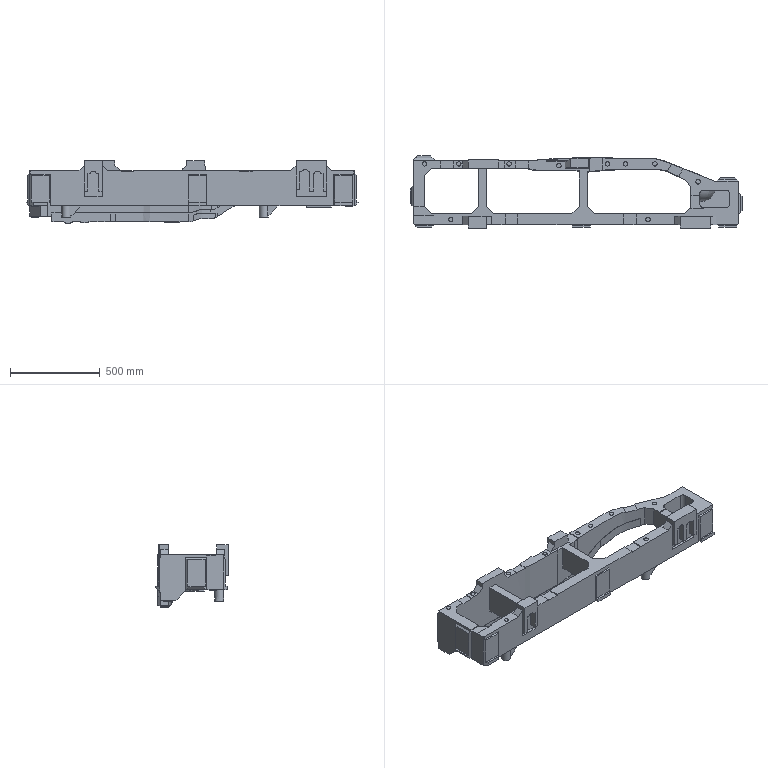Part | NX | features solid 2 | 1 solid | 450 faces | box 1850 x 403.052 x 349.5 mm | volume 58380997 mm3 | plane 238 | spline 176 | cylinder 32 | cone 4 | commonest cylinder face diameters 25 x10 40 x8 42 x6 20 x4 50 x2 30 x1